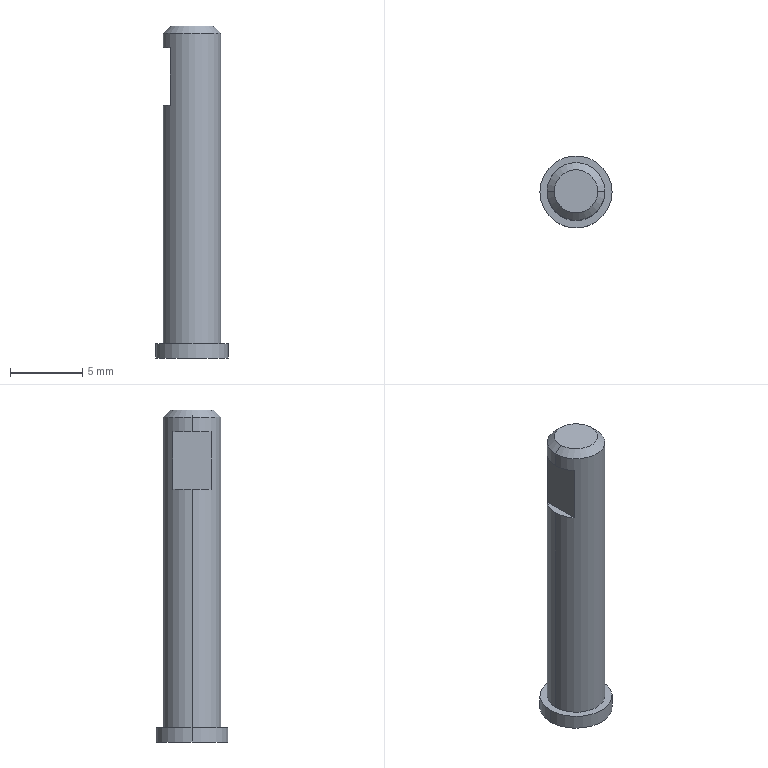Part | STEP file | 2092 Shaft | 1 solid | 12 faces | box 5 x 5 x 23 mm | volume 291.029 mm3 | plane 6 | cylinder 4 | cone 2 | commonest cylinder face diameters 4 x2 5 x2
STEP:
#1=CARTESIAN_POINT('',(0.,0.,0.));
#2=DIRECTION('',(0.,0.,1.));
#3=DIRECTION('',(1.,0.,0.));
#4=AXIS2_PLACEMENT_3D('',#1,#2,#3);
#5=CARTESIAN_POINT('',(1.5,0.,23.));
#6=VERTEX_POINT('',#5);
#7=CARTESIAN_POINT('',(-1.5,0.,23.));
#8=VERTEX_POINT('',#7);
#9=CARTESIAN_POINT('',(0.,0.,23.));
#10=DIRECTION('',(0.,0.,1.));
#11=DIRECTION('',(1.,0.,0.));
#12=AXIS2_PLACEMENT_3D('',#9,#10,#11);
#13=CIRCLE('',#12,1.5);
#14=CARTESIAN_POINT('',(0.,0.,23.));
#15=DIRECTION('',(0.,0.,-1.));
#16=DIRECTION('',(-1.,0.,0.));
#17=AXIS2_PLACEMENT_3D('',#14,#15,#16);
#18=CONICAL_SURFACE('',#17,1.5,0.7854);
#19=CARTESIAN_POINT('',(3.142,0.));
#20=DIRECTION('',(-1.,0.));
#21=VECTOR('',#20,1.);
#22=LINE('',#19,#21);
#23=(GEOMETRIC_REPRESENTATION_CONTEXT(2)PARAMETRIC_REPRESENTATION_CONTEXT()REPRESENTATION_CONTEXT('',''));
#24=DEFINITIONAL_REPRESENTATION('',(#22),#23);
#25=PCURVE('',#18,#24);
#26=CARTESIAN_POINT('',(0.,0.,23.));
#27=DIRECTION('',(0.,0.,1.));
#28=DIRECTION('',(1.,0.,0.));
#29=AXIS2_PLACEMENT_3D('',#26,#27,#28);
#30=PLANE('',#29);
#31=CARTESIAN_POINT('',(0.,0.));
#32=DIRECTION('',(1.,0.));
#33=AXIS2_PLACEMENT_2D('',#31,#32);
#34=CIRCLE('',#33,1.5);
#35=(GEOMETRIC_REPRESENTATION_CONTEXT(2)PARAMETRIC_REPRESENTATION_CONTEXT()REPRESENTATION_CONTEXT('',''));
#36=DEFINITIONAL_REPRESENTATION('',(#34),#35);
#37=PCURVE('',#30,#36);
#38=SURFACE_CURVE('',#13,(#25,#37),.PCURVE_S1.);
#39=EDGE_CURVE('',#6,#8,#38,.T.);
#40=ORIENTED_EDGE('',*,*,#39,.F.);
#41=CARTESIAN_POINT('',(2.,0.,22.5));
#42=VERTEX_POINT('',#41);
#43=CARTESIAN_POINT('',(1.5,0.,23.));
#44=DIRECTION('',(0.7071,0.,-0.7071));
#45=VECTOR('',#44,1.);
#46=LINE('',#43,#45);
#47=CARTESIAN_POINT('',(3.142,0.));
#48=DIRECTION('',(0.,1.));
#49=VECTOR('',#48,1.);
#50=LINE('',#47,#49);
#51=(GEOMETRIC_REPRESENTATION_CONTEXT(2)PARAMETRIC_REPRESENTATION_CONTEXT()REPRESENTATION_CONTEXT('',''));
#52=DEFINITIONAL_REPRESENTATION('',(#50),#51);
#53=PCURVE('',#18,#52);
#54=CARTESIAN_POINT('',(0.,0.,23.));
#55=DIRECTION('',(0.,0.,-1.));
#56=DIRECTION('',(-1.,0.,0.));
#57=AXIS2_PLACEMENT_3D('',#54,#55,#56);
#58=CONICAL_SURFACE('',#57,1.5,0.7854);
#59=CARTESIAN_POINT('',(3.142,0.));
#60=DIRECTION('',(0.,1.));
#61=VECTOR('',#60,1.);
#62=LINE('',#59,#61);
#63=(GEOMETRIC_REPRESENTATION_CONTEXT(2)PARAMETRIC_REPRESENTATION_CONTEXT()REPRESENTATION_CONTEXT('',''));
#64=DEFINITIONAL_REPRESENTATION('',(#62),#63);
#65=PCURVE('',#58,#64);
#66=SURFACE_CURVE('',#46,(#53,#65),.PCURVE_S1.);
#67=EDGE_CURVE('',#6,#42,#66,.T.);
#68=ORIENTED_EDGE('',*,*,#67,.T.);
#69=CARTESIAN_POINT('',(-2.,0.,22.5));
#70=VERTEX_POINT('',#69);
#71=CARTESIAN_POINT('',(0.,0.,22.5));
#72=DIRECTION('',(0.,0.,-1.));
#73=DIRECTION('',(1.,0.,0.));
#74=AXIS2_PLACEMENT_3D('',#71,#72,#73);
#75=CIRCLE('',#74,2.);
#76=CARTESIAN_POINT('',(-3.142,0.5));
#77=DIRECTION('',(1.,0.));
#78=VECTOR('',#77,1.);
#79=LINE('',#76,#78);
#80=(GEOMETRIC_REPRESENTATION_CONTEXT(2)PARAMETRIC_REPRESENTATION_CONTEXT()REPRESENTATION_CONTEXT('',''));
#81=DEFINITIONAL_REPRESENTATION('',(#79),#80);
#82=PCURVE('',#18,#81);
#83=CARTESIAN_POINT('',(0.,0.,23.));
#84=DIRECTION('',(0.,0.,-1.));
#85=DIRECTION('',(-1.,0.,0.));
#86=AXIS2_PLACEMENT_3D('',#83,#84,#85);
#87=CYLINDRICAL_SURFACE('',#86,2.);
#88=CARTESIAN_POINT('',(-3.142,0.5));
#89=DIRECTION('',(1.,0.));
#90=VECTOR('',#89,1.);
#91=LINE('',#88,#90);
#92=(GEOMETRIC_REPRESENTATION_CONTEXT(2)PARAMETRIC_REPRESENTATION_CONTEXT()REPRESENTATION_CONTEXT('',''));
#93=DEFINITIONAL_REPRESENTATION('',(#91),#92);
#94=PCURVE('',#87,#93);
#95=SURFACE_CURVE('',#75,(#82,#94),.PCURVE_S1.);
#96=EDGE_CURVE('',#70,#42,#95,.T.);
#97=ORIENTED_EDGE('',*,*,#96,.F.);
#98=CARTESIAN_POINT('',(-1.5,0.,23.));
#99=DIRECTION('',(-0.7071,0.,-0.7071));
#100=VECTOR('',#99,1.);
#101=LINE('',#98,#100);
#102=CARTESIAN_POINT('',(0.,0.));
#103=DIRECTION('',(0.,1.));
#104=VECTOR('',#103,1.);
#105=LINE('',#102,#104);
#106=(GEOMETRIC_REPRESENTATION_CONTEXT(2)PARAMETRIC_REPRESENTATION_CONTEXT()REPRESENTATION_CONTEXT('',''));
#107=DEFINITIONAL_REPRESENTATION('',(#105),#106);
#108=PCURVE('',#18,#107);
#109=CARTESIAN_POINT('',(6.283,0.));
#110=DIRECTION('',(0.,1.));
#111=VECTOR('',#110,1.);
#112=LINE('',#109,#111);
#113=(GEOMETRIC_REPRESENTATION_CONTEXT(2)PARAMETRIC_REPRESENTATION_CONTEXT()REPRESENTATION_CONTEXT('',''));
#114=DEFINITIONAL_REPRESENTATION('',(#112),#113);
#115=PCURVE('',#58,#114);
#116=SURFACE_CURVE('',#101,(#108,#115),.PCURVE_S1.);
#117=EDGE_CURVE('',#8,#70,#116,.T.);
#118=ORIENTED_EDGE('',*,*,#117,.F.);
#119=EDGE_LOOP('',(#40,#68,#97,#118));
#120=FACE_BOUND('',#119,.T.);
#121=ADVANCED_FACE('',(#120),#18,.T.);
#122=CARTESIAN_POINT('',(2.5,0.,1.));
#123=VERTEX_POINT('',#122);
#124=CARTESIAN_POINT('',(-2.5,0.,1.));
#125=VERTEX_POINT('',#124);
#126=CARTESIAN_POINT('',(0.,0.,1.));
#127=DIRECTION('',(0.,0.,1.));
#128=DIRECTION('',(1.,0.,0.));
#129=AXIS2_PLACEMENT_3D('',#126,#127,#128);
#130=CIRCLE('',#129,2.5);
#131=CARTESIAN_POINT('',(0.,0.,1.));
#132=DIRECTION('',(0.,0.,-1.));
#133=DIRECTION('',(-1.,0.,0.));
#134=AXIS2_PLACEMENT_3D('',#131,#132,#133);
#135=CYLINDRICAL_SURFACE('',#134,2.5);
#136=CARTESIAN_POINT('',(3.142,0.));
#137=DIRECTION('',(-1.,0.));
#138=VECTOR('',#137,1.);
#139=LINE('',#136,#138);
#140=(GEOMETRIC_REPRESENTATION_CONTEXT(2)PARAMETRIC_REPRESENTATION_CONTEXT()REPRESENTATION_CONTEXT('',''));
#141=DEFINITIONAL_REPRESENTATION('',(#139),#140);
#142=PCURVE('',#135,#141);
#143=CARTESIAN_POINT('',(0.,0.,1.));
#144=DIRECTION('',(0.,0.,1.));
#145=DIRECTION('',(1.,0.,0.));
#146=AXIS2_PLACEMENT_3D('',#143,#144,#145);
#147=PLANE('',#146);
#148=CARTESIAN_POINT('',(0.,0.));
#149=DIRECTION('',(1.,0.));
#150=AXIS2_PLACEMENT_2D('',#148,#149);
#151=CIRCLE('',#150,2.5);
#152=(GEOMETRIC_REPRESENTATION_CONTEXT(2)PARAMETRIC_REPRESENTATION_CONTEXT()REPRESENTATION_CONTEXT('',''));
#153=DEFINITIONAL_REPRESENTATION('',(#151),#152);
#154=PCURVE('',#147,#153);
#155=SURFACE_CURVE('',#130,(#142,#154),.PCURVE_S1.);
#156=EDGE_CURVE('',#123,#125,#155,.T.);
#157=ORIENTED_EDGE('',*,*,#156,.F.);
#158=CARTESIAN_POINT('',(2.5,0.,0.));
#159=VERTEX_POINT('',#158);
#160=CARTESIAN_POINT('',(2.5,0.,1.));
#161=DIRECTION('',(0.,0.,-1.));
#162=VECTOR('',#161,1.);
#163=LINE('',#160,#162);
#164=CARTESIAN_POINT('',(3.142,0.));
#165=DIRECTION('',(0.,1.));
#166=VECTOR('',#165,1.);
#167=LINE('',#164,#166);
#168=(GEOMETRIC_REPRESENTATION_CONTEXT(2)PARAMETRIC_REPRESENTATION_CONTEXT()REPRESENTATION_CONTEXT('',''));
#169=DEFINITIONAL_REPRESENTATION('',(#167),#168);
#170=PCURVE('',#135,#169);
#171=CARTESIAN_POINT('',(0.,0.,1.));
#172=DIRECTION('',(0.,0.,-1.));
#173=DIRECTION('',(-1.,0.,0.));
#174=AXIS2_PLACEMENT_3D('',#171,#172,#173);
#175=CYLINDRICAL_SURFACE('',#174,2.5);
#176=CARTESIAN_POINT('',(3.142,0.));
#177=DIRECTION('',(0.,1.));
#178=VECTOR('',#177,1.);
#179=LINE('',#176,#178);
#180=(GEOMETRIC_REPRESENTATION_CONTEXT(2)PARAMETRIC_REPRESENTATION_CONTEXT()REPRESENTATION_CONTEXT('',''));
#181=DEFINITIONAL_REPRESENTATION('',(#179),#180);
#182=PCURVE('',#175,#181);
#183=SURFACE_CURVE('',#163,(#170,#182),.PCURVE_S1.);
#184=EDGE_CURVE('',#123,#159,#183,.T.);
#185=ORIENTED_EDGE('',*,*,#184,.T.);
#186=CARTESIAN_POINT('',(-2.5,0.,0.));
#187=VERTEX_POINT('',#186);
#188=CARTESIAN_POINT('',(0.,0.,0.));
#189=DIRECTION('',(0.,0.,1.));
#190=DIRECTION('',(1.,0.,0.));
#191=AXIS2_PLACEMENT_3D('',#188,#189,#190);
#192=CIRCLE('',#191,2.5);
#193=CARTESIAN_POINT('',(3.142,1.));
#194=DIRECTION('',(-1.,0.));
#195=VECTOR('',#194,1.);
#196=LINE('',#193,#195);
#197=(GEOMETRIC_REPRESENTATION_CONTEXT(2)PARAMETRIC_REPRESENTATION_CONTEXT()REPRESENTATION_CONTEXT('',''));
#198=DEFINITIONAL_REPRESENTATION('',(#196),#197);
#199=PCURVE('',#135,#198);
#200=CARTESIAN_POINT('',(0.,0.,0.));
#201=DIRECTION('',(0.,0.,1.));
#202=DIRECTION('',(1.,0.,0.));
#203=AXIS2_PLACEMENT_3D('',#200,#201,#202);
#204=PLANE('',#203);
#205=CARTESIAN_POINT('',(0.,0.));
#206=DIRECTION('',(1.,0.));
#207=AXIS2_PLACEMENT_2D('',#205,#206);
#208=CIRCLE('',#207,2.5);
#209=(GEOMETRIC_REPRESENTATION_CONTEXT(2)PARAMETRIC_REPRESENTATION_CONTEXT()REPRESENTATION_CONTEXT('',''));
#210=DEFINITIONAL_REPRESENTATION('',(#208),#209);
#211=PCURVE('',#204,#210);
#212=SURFACE_CURVE('',#192,(#199,#211),.PCURVE_S1.);
#213=EDGE_CURVE('',#159,#187,#212,.T.);
#214=ORIENTED_EDGE('',*,*,#213,.T.);
#215=CARTESIAN_POINT('',(-2.5,0.,1.));
#216=DIRECTION('',(0.,0.,-1.));
#217=VECTOR('',#216,1.);
#218=LINE('',#215,#217);
#219=CARTESIAN_POINT('',(0.,0.));
#220=DIRECTION('',(0.,1.));
#221=VECTOR('',#220,1.);
#222=LINE('',#219,#221);
#223=(GEOMETRIC_REPRESENTATION_CONTEXT(2)PARAMETRIC_REPRESENTATION_CONTEXT()REPRESENTATION_CONTEXT('',''));
#224=DEFINITIONAL_REPRESENTATION('',(#222),#223);
#225=PCURVE('',#135,#224);
#226=CARTESIAN_POINT('',(6.283,0.));
#227=DIRECTION('',(0.,1.));
#228=VECTOR('',#227,1.);
#229=LINE('',#226,#228);
#230=(GEOMETRIC_REPRESENTATION_CONTEXT(2)PARAMETRIC_REPRESENTATION_CONTEXT()REPRESENTATION_CONTEXT('',''));
#231=DEFINITIONAL_REPRESENTATION('',(#229),#230);
#232=PCURVE('',#175,#231);
#233=SURFACE_CURVE('',#218,(#225,#232),.PCURVE_S1.);
#234=EDGE_CURVE('',#125,#187,#233,.T.);
#235=ORIENTED_EDGE('',*,*,#234,.F.);
#236=EDGE_LOOP('',(#157,#185,#214,#235));
#237=FACE_BOUND('',#236,.T.);
#238=ADVANCED_FACE('',(#237),#135,.T.);
#239=ORIENTED_EDGE('',*,*,#96,.T.);
#240=CARTESIAN_POINT('',(2.,0.,1.));
#241=VERTEX_POINT('',#240);
#242=CARTESIAN_POINT('',(2.,0.,23.));
#243=DIRECTION('',(0.,0.,-1.));
#244=VECTOR('',#243,1.);
#245=LINE('',#242,#244);
#246=CARTESIAN_POINT('',(3.142,0.));
#247=DIRECTION('',(0.,1.));
#248=VECTOR('',#247,1.);
#249=LINE('',#246,#248);
#250=(GEOMETRIC_REPRESENTATION_CONTEXT(2)PARAMETRIC_REPRESENTATION_CONTEXT()REPRESENTATION_CONTEXT('',''));
#251=DEFINITIONAL_REPRESENTATION('',(#249),#250);
#252=PCURVE('',#87,#251);
#253=CARTESIAN_POINT('',(0.,0.,23.));
#254=DIRECTION('',(0.,0.,-1.));
#255=DIRECTION('',(-1.,0.,0.));
#256=AXIS2_PLACEMENT_3D('',#253,#254,#255);
#257=CYLINDRICAL_SURFACE('',#256,2.);
#258=CARTESIAN_POINT('',(3.142,0.));
#259=DIRECTION('',(0.,1.));
#260=VECTOR('',#259,1.);
#261=LINE('',#258,#260);
#262=(GEOMETRIC_REPRESENTATION_CONTEXT(2)PARAMETRIC_REPRESENTATION_CONTEXT()REPRESENTATION_CONTEXT('',''));
#263=DEFINITIONAL_REPRESENTATION('',(#261),#262);
#264=PCURVE('',#257,#263);
#265=SURFACE_CURVE('',#245,(#252,#264),.PCURVE_S1.);
#266=EDGE_CURVE('',#42,#241,#265,.T.);
#267=ORIENTED_EDGE('',*,*,#266,.T.);
#268=CARTESIAN_POINT('',(-2.,0.,1.));
#269=VERTEX_POINT('',#268);
#270=CARTESIAN_POINT('',(0.,0.,1.));
#271=DIRECTION('',(0.,0.,1.));
#272=DIRECTION('',(1.,0.,0.));
#273=AXIS2_PLACEMENT_3D('',#270,#271,#272);
#274=CIRCLE('',#273,2.);
#275=CARTESIAN_POINT('',(3.142,22.));
#276=DIRECTION('',(-1.,0.));
#277=VECTOR('',#276,1.);
#278=LINE('',#275,#277);
#279=(GEOMETRIC_REPRESENTATION_CONTEXT(2)PARAMETRIC_REPRESENTATION_CONTEXT()REPRESENTATION_CONTEXT('',''));
#280=DEFINITIONAL_REPRESENTATION('',(#278),#279);
#281=PCURVE('',#87,#280);
#282=CARTESIAN_POINT('',(0.,0.));
#283=DIRECTION('',(1.,0.));
#284=AXIS2_PLACEMENT_2D('',#282,#283);
#285=CIRCLE('',#284,2.);
#286=(GEOMETRIC_REPRESENTATION_CONTEXT(2)PARAMETRIC_REPRESENTATION_CONTEXT()REPRESENTATION_CONTEXT('',''));
#287=DEFINITIONAL_REPRESENTATION('',(#285),#286);
#288=PCURVE('',#147,#287);
#289=SURFACE_CURVE('',#274,(#281,#288),.PCURVE_S1.);
#290=EDGE_CURVE('',#241,#269,#289,.T.);
#291=ORIENTED_EDGE('',*,*,#290,.T.);
#292=CARTESIAN_POINT('',(-2.,0.,17.5));
#293=VERTEX_POINT('',#292);
#294=CARTESIAN_POINT('',(-2.,0.,23.));
#295=DIRECTION('',(0.,0.,-1.));
#296=VECTOR('',#295,1.);
#297=LINE('',#294,#296);
#298=CARTESIAN_POINT('',(0.,0.));
#299=DIRECTION('',(0.,1.));
#300=VECTOR('',#299,1.);
#301=LINE('',#298,#300);
#302=(GEOMETRIC_REPRESENTATION_CONTEXT(2)PARAMETRIC_REPRESENTATION_CONTEXT()REPRESENTATION_CONTEXT('',''));
#303=DEFINITIONAL_REPRESENTATION('',(#301),#302);
#304=PCURVE('',#87,#303);
#305=CARTESIAN_POINT('',(6.283,0.));
#306=DIRECTION('',(0.,1.));
#307=VECTOR('',#306,1.);
#308=LINE('',#305,#307);
#309=(GEOMETRIC_REPRESENTATION_CONTEXT(2)PARAMETRIC_REPRESENTATION_CONTEXT()REPRESENTATION_CONTEXT('',''));
#310=DEFINITIONAL_REPRESENTATION('',(#308),#309);
#311=PCURVE('',#257,#310);
#312=SURFACE_CURVE('',#297,(#304,#311),.PCURVE_S1.);
#313=EDGE_CURVE('',#293,#269,#312,.T.);
#314=ORIENTED_EDGE('',*,*,#313,.F.);
#315=CARTESIAN_POINT('',(-1.5,1.323,17.5));
#316=VERTEX_POINT('',#315);
#317=CARTESIAN_POINT('',(0.,0.,17.5));
#318=DIRECTION('',(0.,0.,1.));
#319=DIRECTION('',(1.,0.,0.));
#320=AXIS2_PLACEMENT_3D('',#317,#318,#319);
#321=CIRCLE('',#320,2.);
#322=CARTESIAN_POINT('',(3.142,5.5));
#323=DIRECTION('',(-1.,0.));
#324=VECTOR('',#323,1.);
#325=LINE('',#322,#324);
#326=(GEOMETRIC_REPRESENTATION_CONTEXT(2)PARAMETRIC_REPRESENTATION_CONTEXT()REPRESENTATION_CONTEXT('',''));
#327=DEFINITIONAL_REPRESENTATION('',(#325),#326);
#328=PCURVE('',#87,#327);
#329=CARTESIAN_POINT('',(-5.215,6.,17.5));
#330=DIRECTION('',(0.,0.,1.));
#331=DIRECTION('',(1.,0.,0.));
#332=AXIS2_PLACEMENT_3D('',#329,#330,#331);
#333=PLANE('',#332);
#334=CARTESIAN_POINT('',(5.215,-6.));
#335=DIRECTION('',(1.,0.));
#336=AXIS2_PLACEMENT_2D('',#334,#335);
#337=CIRCLE('',#336,2.);
#338=(GEOMETRIC_REPRESENTATION_CONTEXT(2)PARAMETRIC_REPRESENTATION_CONTEXT()REPRESENTATION_CONTEXT('',''));
#339=DEFINITIONAL_REPRESENTATION('',(#337),#338);
#340=PCURVE('',#333,#339);
#341=SURFACE_CURVE('',#321,(#328,#340),.PCURVE_S1.);
#342=EDGE_CURVE('',#316,#293,#341,.T.);
#343=ORIENTED_EDGE('',*,*,#342,.F.);
#344=CARTESIAN_POINT('',(-1.5,1.323,21.5));
#345=VERTEX_POINT('',#344);
#346=CARTESIAN_POINT('',(-1.5,1.323,23.));
#347=DIRECTION('',(0.,0.,-1.));
#348=VECTOR('',#347,1.);
#349=LINE('',#346,#348);
#350=CARTESIAN_POINT('',(0.7227,0.));
#351=DIRECTION('',(0.,1.));
#352=VECTOR('',#351,1.);
#353=LINE('',#350,#352);
#354=(GEOMETRIC_REPRESENTATION_CONTEXT(2)PARAMETRIC_REPRESENTATION_CONTEXT()REPRESENTATION_CONTEXT('',''));
#355=DEFINITIONAL_REPRESENTATION('',(#353),#354);
#356=PCURVE('',#87,#355);
#357=CARTESIAN_POINT('',(-1.5,6.,17.5));
#358=DIRECTION('',(-1.,0.,0.));
#359=DIRECTION('',(0.,0.,1.));
#360=AXIS2_PLACEMENT_3D('',#357,#358,#359);
#361=PLANE('',#360);
#362=CARTESIAN_POINT('',(5.5,-4.677));
#363=DIRECTION('',(-1.,0.));
#364=VECTOR('',#363,1.);
#365=LINE('',#362,#364);
#366=(GEOMETRIC_REPRESENTATION_CONTEXT(2)PARAMETRIC_REPRESENTATION_CONTEXT()REPRESENTATION_CONTEXT('',''));
#367=DEFINITIONAL_REPRESENTATION('',(#365),#366);
#368=PCURVE('',#361,#367);
#369=SURFACE_CURVE('',#349,(#356,#368),.PCURVE_S1.);
#370=EDGE_CURVE('',#345,#316,#369,.T.);
#371=ORIENTED_EDGE('',*,*,#370,.F.);
#372=CARTESIAN_POINT('',(-2.,0.,21.5));
#373=VERTEX_POINT('',#372);
#374=CARTESIAN_POINT('',(0.,0.,21.5));
#375=DIRECTION('',(0.,0.,-1.));
#376=DIRECTION('',(-1.,0.,0.));
#377=AXIS2_PLACEMENT_3D('',#374,#375,#376);
#378=CIRCLE('',#377,2.);
#379=CARTESIAN_POINT('',(0.,1.5));
#380=DIRECTION('',(1.,0.));
#381=VECTOR('',#380,1.);
#382=LINE('',#379,#381);
#383=(GEOMETRIC_REPRESENTATION_CONTEXT(2)PARAMETRIC_REPRESENTATION_CONTEXT()REPRESENTATION_CONTEXT('',''));
#384=DEFINITIONAL_REPRESENTATION('',(#382),#383);
#385=PCURVE('',#87,#384);
#386=CARTESIAN_POINT('',(-5.215,6.,21.5));
#387=DIRECTION('',(0.,0.,-1.));
#388=DIRECTION('',(-1.,0.,0.));
#389=AXIS2_PLACEMENT_3D('',#386,#387,#388);
#390=PLANE('',#389);
#391=CARTESIAN_POINT('',(-5.215,-6.));
#392=DIRECTION('',(1.,0.));
#393=AXIS2_PLACEMENT_2D('',#391,#392);
#394=CIRCLE('',#393,2.);
#395=(GEOMETRIC_REPRESENTATION_CONTEXT(2)PARAMETRIC_REPRESENTATION_CONTEXT()REPRESENTATION_CONTEXT('',''));
#396=DEFINITIONAL_REPRESENTATION('',(#394),#395);
#397=PCURVE('',#390,#396);
#398=SURFACE_CURVE('',#378,(#385,#397),.PCURVE_S1.);
#399=EDGE_CURVE('',#373,#345,#398,.T.);
#400=ORIENTED_EDGE('',*,*,#399,.F.);
#401=CARTESIAN_POINT('',(-2.,0.,23.));
#402=DIRECTION('',(0.,0.,-1.));
#403=VECTOR('',#402,1.);
#404=LINE('',#401,#403);
#405=CARTESIAN_POINT('',(0.,0.));
#406=DIRECTION('',(0.,1.));
#407=VECTOR('',#406,1.);
#408=LINE('',#405,#407);
#409=(GEOMETRIC_REPRESENTATION_CONTEXT(2)PARAMETRIC_REPRESENTATION_CONTEXT()REPRESENTATION_CONTEXT('',''));
#410=DEFINITIONAL_REPRESENTATION('',(#408),#409);
#411=PCURVE('',#87,#410);
#412=CARTESIAN_POINT('',(6.283,0.));
#413=DIRECTION('',(0.,1.));
#414=VECTOR('',#413,1.);
#415=LINE('',#412,#414);
#416=(GEOMETRIC_REPRESENTATION_CONTEXT(2)PARAMETRIC_REPRESENTATION_CONTEXT()REPRESENTATION_CONTEXT('',''));
#417=DEFINITIONAL_REPRESENTATION('',(#415),#416);
#418=PCURVE('',#257,#417);
#419=SURFACE_CURVE('',#404,(#411,#418),.PCURVE_S1.);
#420=EDGE_CURVE('',#70,#373,#419,.T.);
#421=ORIENTED_EDGE('',*,*,#420,.F.);
#422=EDGE_LOOP('',(#239,#267,#291,#314,#343,#371,#400,#421));
#423=FACE_BOUND('',#422,.T.);
#424=ADVANCED_FACE('',(#423),#87,.T.);
#425=ORIENTED_EDGE('',*,*,#266,.F.);
#426=CARTESIAN_POINT('',(0.,0.,22.5));
#427=DIRECTION('',(0.,0.,-1.));
#428=DIRECTION('',(1.,0.,0.));
#429=AXIS2_PLACEMENT_3D('',#426,#427,#428);
#430=CIRCLE('',#429,2.);
#431=CARTESIAN_POINT('',(3.142,0.5));
#432=DIRECTION('',(1.,0.));
#433=VECTOR('',#432,1.);
#434=LINE('',#431,#433);
#435=(GEOMETRIC_REPRESENTATION_CONTEXT(2)PARAMETRIC_REPRESENTATION_CONTEXT()REPRESENTATION_CONTEXT('',''));
#436=DEFINITIONAL_REPRESENTATION('',(#434),#435);
#437=PCURVE('',#257,#436);
#438=CARTESIAN_POINT('',(3.142,0.5));
#439=DIRECTION('',(1.,0.));
#440=VECTOR('',#439,1.);
#441=LINE('',#438,#440);
#442=(GEOMETRIC_REPRESENTATION_CONTEXT(2)PARAMETRIC_REPRESENTATION_CONTEXT()REPRESENTATION_CONTEXT('',''));
#443=DEFINITIONAL_REPRESENTATION('',(#441),#442);
#444=PCURVE('',#58,#443);
#445=SURFACE_CURVE('',#430,(#437,#444),.PCURVE_S1.);
#446=EDGE_CURVE('',#42,#70,#445,.T.);
#447=ORIENTED_EDGE('',*,*,#446,.T.);
#448=ORIENTED_EDGE('',*,*,#420,.T.);
#449=CARTESIAN_POINT('',(-1.5,-1.323,21.5));
#450=VERTEX_POINT('',#449);
#451=CARTESIAN_POINT('',(0.,0.,21.5));
#452=DIRECTION('',(0.,0.,-1.));
#453=DIRECTION('',(-1.,0.,0.));
#454=AXIS2_PLACEMENT_3D('',#451,#452,#453);
#455=CIRCLE('',#454,2.);
#456=CARTESIAN_POINT('',(0.,1.5));
#457=DIRECTION('',(1.,0.));
#458=VECTOR('',#457,1.);
#459=LINE('',#456,#458);
#460=(GEOMETRIC_REPRESENTATION_CONTEXT(2)PARAMETRIC_REPRESENTATION_CONTEXT()REPRESENTATION_CONTEXT('',''));
#461=DEFINITIONAL_REPRESENTATION('',(#459),#460);
#462=PCURVE('',#257,#461);
#463=CARTESIAN_POINT('',(-5.215,-6.));
#464=DIRECTION('',(1.,0.));
#465=AXIS2_PLACEMENT_2D('',#463,#464);
#466=CIRCLE('',#465,2.);
#467=(GEOMETRIC_REPRESENTATION_CONTEXT(2)PARAMETRIC_REPRESENTATION_CONTEXT()REPRESENTATION_CONTEXT('',''));
#468=DEFINITIONAL_REPRESENTATION('',(#466),#467);
#469=PCURVE('',#390,#468);
#470=SURFACE_CURVE('',#455,(#462,#469),.PCURVE_S1.);
#471=EDGE_CURVE('',#450,#373,#470,.T.);
#472=ORIENTED_EDGE('',*,*,#471,.F.);
#473=CARTESIAN_POINT('',(-1.5,-1.323,17.5));
#474=VERTEX_POINT('',#473);
#475=CARTESIAN_POINT('',(-1.5,-1.323,23.));
#476=DIRECTION('',(0.,0.,1.));
#477=VECTOR('',#476,1.);
#478=LINE('',#475,#477);
#479=CARTESIAN_POINT('',(5.56,0.));
#480=DIRECTION('',(0.,-1.));
#481=VECTOR('',#480,1.);
#482=LINE('',#479,#481);
#483=(GEOMETRIC_REPRESENTATION_CONTEXT(2)PARAMETRIC_REPRESENTATION_CONTEXT()REPRESENTATION_CONTEXT('',''));
#484=DEFINITIONAL_REPRESENTATION('',(#482),#483);
#485=PCURVE('',#257,#484);
#486=CARTESIAN_POINT('',(5.5,-7.323));
#487=DIRECTION('',(1.,0.));
#488=VECTOR('',#487,1.);
#489=LINE('',#486,#488);
#490=(GEOMETRIC_REPRESENTATION_CONTEXT(2)PARAMETRIC_REPRESENTATION_CONTEXT()REPRESENTATION_CONTEXT('',''));
#491=DEFINITIONAL_REPRESENTATION('',(#489),#490);
#492=PCURVE('',#361,#491);
#493=SURFACE_CURVE('',#478,(#485,#492),.PCURVE_S1.);
#494=EDGE_CURVE('',#474,#450,#493,.T.);
#495=ORIENTED_EDGE('',*,*,#494,.F.);
#496=CARTESIAN_POINT('',(0.,0.,17.5));
#497=DIRECTION('',(0.,0.,1.));
#498=DIRECTION('',(1.,0.,0.));
#499=AXIS2_PLACEMENT_3D('',#496,#497,#498);
#500=CIRCLE('',#499,2.);
#501=CARTESIAN_POINT('',(9.425,5.5));
#502=DIRECTION('',(-1.,0.));
#503=VECTOR('',#502,1.);
#504=LINE('',#501,#503);
#505=(GEOMETRIC_REPRESENTATION_CONTEXT(2)PARAMETRIC_REPRESENTATION_CONTEXT()REPRESENTATION_CONTEXT('',''));
#506=DEFINITIONAL_REPRESENTATION('',(#504),#505);
#507=PCURVE('',#257,#506);
#508=CARTESIAN_POINT('',(5.215,-6.));
#509=DIRECTION('',(1.,0.));
#510=AXIS2_PLACEMENT_2D('',#508,#509);
#511=CIRCLE('',#510,2.);
#512=(GEOMETRIC_REPRESENTATION_CONTEXT(2)PARAMETRIC_REPRESENTATION_CONTEXT()REPRESENTATION_CONTEXT('',''));
#513=DEFINITIONAL_REPRESENTATION('',(#511),#512);
#514=PCURVE('',#333,#513);
#515=SURFACE_CURVE('',#500,(#507,#514),.PCURVE_S1.);
#516=EDGE_CURVE('',#293,#474,#515,.T.);
#517=ORIENTED_EDGE('',*,*,#516,.F.);
#518=ORIENTED_EDGE('',*,*,#313,.T.);
#519=CARTESIAN_POINT('',(0.,0.,1.));
#520=DIRECTION('',(0.,0.,1.));
#521=DIRECTION('',(1.,0.,0.));
#522=AXIS2_PLACEMENT_3D('',#519,#520,#521);
#523=CIRCLE('',#522,2.);
#524=CARTESIAN_POINT('',(9.425,22.));
#525=DIRECTION('',(-1.,0.));
#526=VECTOR('',#525,1.);
#527=LINE('',#524,#526);
#528=(GEOMETRIC_REPRESENTATION_CONTEXT(2)PARAMETRIC_REPRESENTATION_CONTEXT()REPRESENTATION_CONTEXT('',''));
#529=DEFINITIONAL_REPRESENTATION('',(#527),#528);
#530=PCURVE('',#257,#529);
#531=CARTESIAN_POINT('',(0.,0.));
#532=DIRECTION('',(1.,0.));
#533=AXIS2_PLACEMENT_2D('',#531,#532);
#534=CIRCLE('',#533,2.);
#535=(GEOMETRIC_REPRESENTATION_CONTEXT(2)PARAMETRIC_REPRESENTATION_CONTEXT()REPRESENTATION_CONTEXT('',''));
#536=DEFINITIONAL_REPRESENTATION('',(#534),#535);
#537=PCURVE('',#147,#536);
#538=SURFACE_CURVE('',#523,(#530,#537),.PCURVE_S1.);
#539=EDGE_CURVE('',#269,#241,#538,.T.);
#540=ORIENTED_EDGE('',*,*,#539,.T.);
#541=EDGE_LOOP('',(#425,#447,#448,#472,#495,#517,#518,#540));
#542=FACE_BOUND('',#541,.T.);
#543=ADVANCED_FACE('',(#542),#257,.T.);
#544=CARTESIAN_POINT('',(0.,0.,1.));
#545=DIRECTION('',(0.,0.,1.));
#546=DIRECTION('',(1.,0.,0.));
#547=AXIS2_PLACEMENT_3D('',#544,#545,#546);
#548=CIRCLE('',#547,2.5);
#549=CARTESIAN_POINT('',(0.,0.));
#550=DIRECTION('',(1.,0.));
#551=AXIS2_PLACEMENT_2D('',#549,#550);
#552=CIRCLE('',#551,2.5);
#553=(GEOMETRIC_REPRESENTATION_CONTEXT(2)PARAMETRIC_REPRESENTATION_CONTEXT()REPRESENTATION_CONTEXT('',''));
#554=DEFINITIONAL_REPRESENTATION('',(#552),#553);
#555=PCURVE('',#147,#554);
#556=CARTESIAN_POINT('',(9.425,0.));
#557=DIRECTION('',(-1.,0.));
#558=VECTOR('',#557,1.);
#559=LINE('',#556,#558);
#560=(GEOMETRIC_REPRESENTATION_CONTEXT(2)PARAMETRIC_REPRESENTATION_CONTEXT()REPRESENTATION_CONTEXT('',''));
#561=DEFINITIONAL_REPRESENTATION('',(#559),#560);
#562=PCURVE('',#175,#561);
#563=SURFACE_CURVE('',#548,(#555,#562),.PCURVE_S1.);
#564=EDGE_CURVE('',#125,#123,#563,.T.);
#565=ORIENTED_EDGE('',*,*,#564,.T.);
#566=ORIENTED_EDGE('',*,*,#156,.T.);
#567=EDGE_LOOP('',(#565,#566));
#568=FACE_BOUND('',#567,.T.);
#569=ORIENTED_EDGE('',*,*,#539,.F.);
#570=ORIENTED_EDGE('',*,*,#290,.F.);
#571=EDGE_LOOP('',(#569,#570));
#572=FACE_BOUND('',#571,.T.);
#573=ADVANCED_FACE('',(#568,#572),#147,.T.);
#574=ORIENTED_EDGE('',*,*,#184,.F.);
#575=ORIENTED_EDGE('',*,*,#564,.F.);
#576=ORIENTED_EDGE('',*,*,#234,.T.);
#577=CARTESIAN_POINT('',(0.,0.,0.));
#578=DIRECTION('',(0.,0.,1.));
#579=DIRECTION('',(1.,0.,0.));
#580=AXIS2_PLACEMENT_3D('',#577,#578,#579);
#581=CIRCLE('',#580,2.5);
#582=CARTESIAN_POINT('',(9.425,1.));
#583=DIRECTION('',(-1.,0.));
#584=VECTOR('',#583,1.);
#585=LINE('',#582,#584);
#586=(GEOMETRIC_REPRESENTATION_CONTEXT(2)PARAMETRIC_REPRESENTATION_CONTEXT()REPRESENTATION_CONTEXT('',''));
#587=DEFINITIONAL_REPRESENTATION('',(#585),#586);
#588=PCURVE('',#175,#587);
#589=CARTESIAN_POINT('',(0.,0.));
#590=DIRECTION('',(1.,0.));
#591=AXIS2_PLACEMENT_2D('',#589,#590);
#592=CIRCLE('',#591,2.5);
#593=(GEOMETRIC_REPRESENTATION_CONTEXT(2)PARAMETRIC_REPRESENTATION_CONTEXT()REPRESENTATION_CONTEXT('',''));
#594=DEFINITIONAL_REPRESENTATION('',(#592),#593);
#595=PCURVE('',#204,#594);
#596=SURFACE_CURVE('',#581,(#588,#595),.PCURVE_S1.);
#597=EDGE_CURVE('',#187,#159,#596,.T.);
#598=ORIENTED_EDGE('',*,*,#597,.T.);
#599=EDGE_LOOP('',(#574,#575,#576,#598));
#600=FACE_BOUND('',#599,.T.);
#601=ADVANCED_FACE('',(#600),#175,.T.);
#602=ORIENTED_EDGE('',*,*,#597,.F.);
#603=ORIENTED_EDGE('',*,*,#213,.F.);
#604=EDGE_LOOP('',(#602,#603));
#605=FACE_BOUND('',#604,.T.);
#606=ADVANCED_FACE('',(#605),#204,.F.);
#607=CARTESIAN_POINT('',(0.,0.,23.));
#608=DIRECTION('',(0.,0.,1.));
#609=DIRECTION('',(1.,0.,0.));
#610=AXIS2_PLACEMENT_3D('',#607,#608,#609);
#611=CIRCLE('',#610,1.5);
#612=CARTESIAN_POINT('',(0.,0.));
#613=DIRECTION('',(1.,0.));
#614=AXIS2_PLACEMENT_2D('',#612,#613);
#615=CIRCLE('',#614,1.5);
#616=(GEOMETRIC_REPRESENTATION_CONTEXT(2)PARAMETRIC_REPRESENTATION_CONTEXT()REPRESENTATION_CONTEXT('',''));
#617=DEFINITIONAL_REPRESENTATION('',(#615),#616);
#618=PCURVE('',#30,#617);
#619=CARTESIAN_POINT('',(9.425,0.));
#620=DIRECTION('',(-1.,0.));
#621=VECTOR('',#620,1.);
#622=LINE('',#619,#621);
#623=(GEOMETRIC_REPRESENTATION_CONTEXT(2)PARAMETRIC_REPRESENTATION_CONTEXT()REPRESENTATION_CONTEXT('',''));
#624=DEFINITIONAL_REPRESENTATION('',(#622),#623);
#625=PCURVE('',#58,#624);
#626=SURFACE_CURVE('',#611,(#618,#625),.PCURVE_S1.);
#627=EDGE_CURVE('',#8,#6,#626,.T.);
#628=ORIENTED_EDGE('',*,*,#627,.T.);
#629=ORIENTED_EDGE('',*,*,#39,.T.);
#630=EDGE_LOOP('',(#628,#629));
#631=FACE_BOUND('',#630,.T.);
#632=ADVANCED_FACE('',(#631),#30,.T.);
#633=ORIENTED_EDGE('',*,*,#471,.T.);
#634=ORIENTED_EDGE('',*,*,#399,.T.);
#635=CARTESIAN_POINT('',(-1.5,6.,21.5));
#636=DIRECTION('',(0.,-1.,0.));
#637=VECTOR('',#636,1.);
#638=LINE('',#635,#637);
#639=CARTESIAN_POINT('',(-3.715,0.));
#640=DIRECTION('',(0.,-1.));
#641=VECTOR('',#640,1.);
#642=LINE('',#639,#641);
#643=(GEOMETRIC_REPRESENTATION_CONTEXT(2)PARAMETRIC_REPRESENTATION_CONTEXT()REPRESENTATION_CONTEXT('',''));
#644=DEFINITIONAL_REPRESENTATION('',(#642),#643);
#645=PCURVE('',#390,#644);
#646=CARTESIAN_POINT('',(4.,0.));
#647=DIRECTION('',(0.,-1.));
#648=VECTOR('',#647,1.);
#649=LINE('',#646,#648);
#650=(GEOMETRIC_REPRESENTATION_CONTEXT(2)PARAMETRIC_REPRESENTATION_CONTEXT()REPRESENTATION_CONTEXT('',''));
#651=DEFINITIONAL_REPRESENTATION('',(#649),#650);
#652=PCURVE('',#361,#651);
#653=SURFACE_CURVE('',#638,(#645,#652),.PCURVE_S1.);
#654=EDGE_CURVE('',#345,#450,#653,.T.);
#655=ORIENTED_EDGE('',*,*,#654,.T.);
#656=EDGE_LOOP('',(#633,#634,#655));
#657=FACE_BOUND('',#656,.T.);
#658=ADVANCED_FACE('',(#657),#390,.T.);
#659=ORIENTED_EDGE('',*,*,#370,.T.);
#660=CARTESIAN_POINT('',(-1.5,6.,17.5));
#661=DIRECTION('',(0.,-1.,0.));
#662=VECTOR('',#661,1.);
#663=LINE('',#660,#662);
#664=CARTESIAN_POINT('',(0.,0.));
#665=DIRECTION('',(0.,-1.));
#666=VECTOR('',#665,1.);
#667=LINE('',#664,#666);
#668=(GEOMETRIC_REPRESENTATION_CONTEXT(2)PARAMETRIC_REPRESENTATION_CONTEXT()REPRESENTATION_CONTEXT('',''));
#669=DEFINITIONAL_REPRESENTATION('',(#667),#668);
#670=PCURVE('',#361,#669);
#671=CARTESIAN_POINT('',(3.715,0.));
#672=DIRECTION('',(0.,-1.));
#673=VECTOR('',#672,1.);
#674=LINE('',#671,#673);
#675=(GEOMETRIC_REPRESENTATION_CONTEXT(2)PARAMETRIC_REPRESENTATION_CONTEXT()REPRESENTATION_CONTEXT('',''));
#676=DEFINITIONAL_REPRESENTATION('',(#674),#675);
#677=PCURVE('',#333,#676);
#678=SURFACE_CURVE('',#663,(#670,#677),.PCURVE_S1.);
#679=EDGE_CURVE('',#316,#474,#678,.T.);
#680=ORIENTED_EDGE('',*,*,#679,.T.);
#681=ORIENTED_EDGE('',*,*,#494,.T.);
#682=ORIENTED_EDGE('',*,*,#654,.F.);
#683=EDGE_LOOP('',(#659,#680,#681,#682));
#684=FACE_BOUND('',#683,.T.);
#685=ADVANCED_FACE('',(#684),#361,.T.);
#686=ORIENTED_EDGE('',*,*,#342,.T.);
#687=ORIENTED_EDGE('',*,*,#516,.T.);
#688=ORIENTED_EDGE('',*,*,#679,.F.);
#689=EDGE_LOOP('',(#686,#687,#688));
#690=FACE_BOUND('',#689,.T.);
#691=ADVANCED_FACE('',(#690),#333,.T.);
#692=ORIENTED_EDGE('',*,*,#67,.F.);
#693=ORIENTED_EDGE('',*,*,#627,.F.);
#694=ORIENTED_EDGE('',*,*,#117,.T.);
#695=ORIENTED_EDGE('',*,*,#446,.F.);
#696=EDGE_LOOP('',(#692,#693,#694,#695));
#697=FACE_BOUND('',#696,.T.);
#698=ADVANCED_FACE('',(#697),#58,.T.);
#699=CLOSED_SHELL('',(#121,#238,#424,#543,#573,#601,#606,#632,#658,#685,#691,#698));
#700=MANIFOLD_SOLID_BREP('',#699);
#701=(LENGTH_UNIT()NAMED_UNIT(*)SI_UNIT(.MILLI.,.METRE.));
#702=UNCERTAINTY_MEASURE_WITH_UNIT(LENGTH_MEASURE(0.0000001),#701,'','');
#703=(NAMED_UNIT(*)PLANE_ANGLE_UNIT()SI_UNIT($,.RADIAN.));
#704=(NAMED_UNIT(*)SI_UNIT($,.STERADIAN.)SOLID_ANGLE_UNIT());
#705=(GEOMETRIC_REPRESENTATION_CONTEXT(3)GLOBAL_UNCERTAINTY_ASSIGNED_CONTEXT((#702))GLOBAL_UNIT_ASSIGNED_CONTEXT((#701,#703,#704))REPRESENTATION_CONTEXT('',''));
#706=ADVANCED_BREP_SHAPE_REPRESENTATION('',(#4,#700),#705);